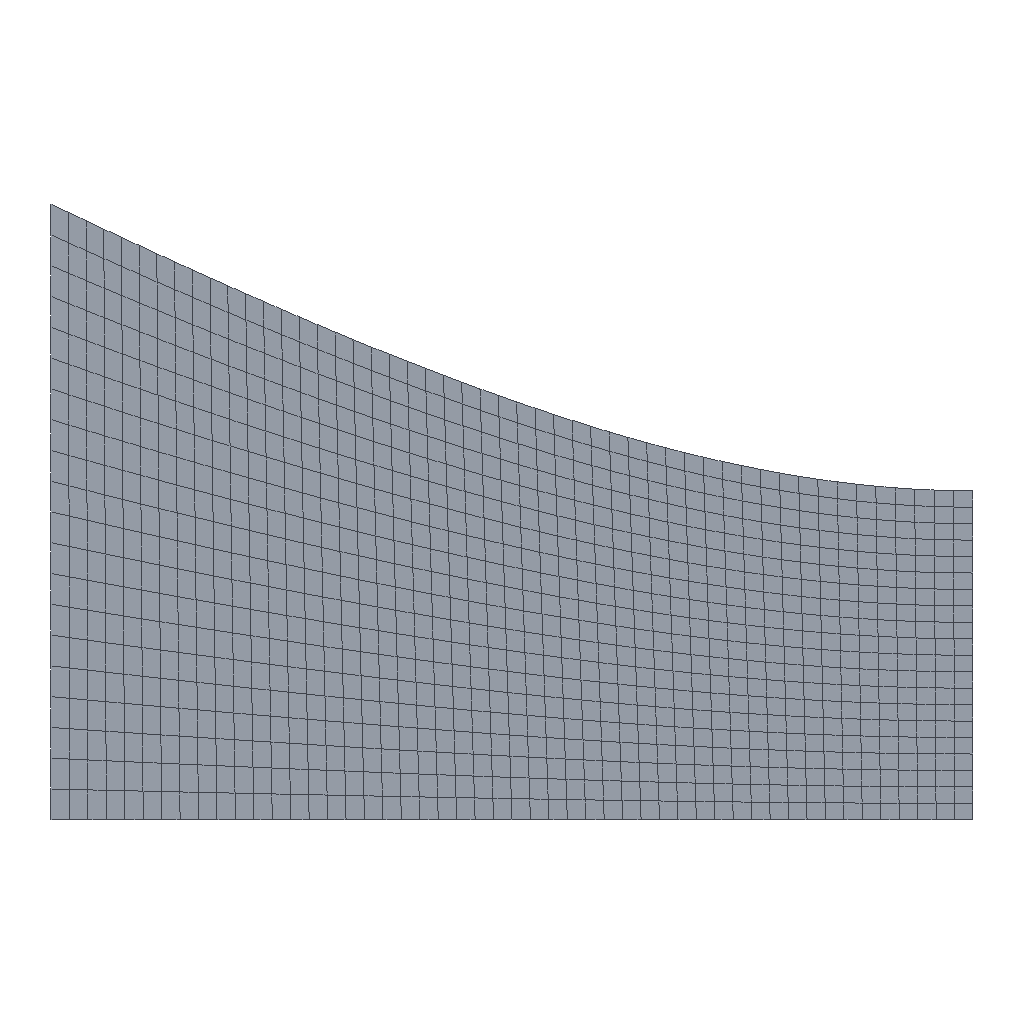Simulation study | ansys fluent
Set-up summary:
category,name,step,type,value,unit,region
solver,ansys_fluent
units,not stated in the deck,,not stated
analysis,deck,,Steady,Steady
physics,Time,,model,Steady
physics,Space,,model,Axisymmetric swirl
physics,Species,,model,Disabled
physics,Viscous,,model,Inviscid
physics,Structure,,model,Disabled
physics,Multiphase,,model,Disabled
physics,Heat Transfer,,model,Enabled
material,aluminum,,solid
material,air,,fluid
bc,in,,pressure-inlet
bc,out,,pressure-outlet
bc,wall,,wall
bc,axis,,axis
Results summary:
result,analysis,,,Steady
result,pressure,,min/max,47736.266 / 100956.86
result,velocity-magnitude,,min/max,25.629 / 341.377
result,temperature,,min/max,242.103 / 299.674